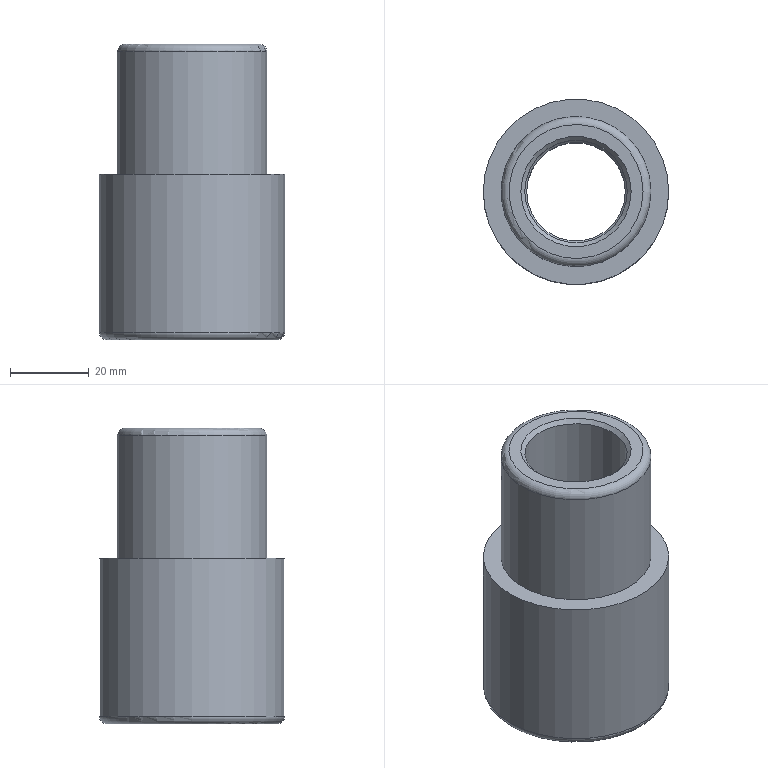Part | NX | features DATUM_CSYS 5, EXTRUDE 4, SKETCH 4, CHAMFER 2, BLEND 1 | 1 solid | 12 faces | box 47 x 47 x 75 mm | volume 71750 mm3 | cylinder 4 | plane 3 | torus 3 | cone 2 | commonest cylinder face diameters 25 x1 26 x1 38 x1 47 x1
STEP:
#1=CARTESIAN_POINT('',(12.5,0.,2.));
#2=VERTEX_POINT('',#1);
#3=CARTESIAN_POINT('',(0.,0.,2.));
#4=DIRECTION('',(0.,0.,1.));
#5=DIRECTION('',(1.,0.,0.));
#6=AXIS2_PLACEMENT_3D('',#3,#4,#5);
#7=CIRCLE('',#6,12.5);
#8=EDGE_CURVE('',#2,#2,#7,.F.);
#9=ORIENTED_EDGE('',*,*,#8,.T.);
#10=EDGE_LOOP('',(#9));
#11=FACE_BOUND('',#10,.T.);
#12=CARTESIAN_POINT('',(12.5,0.,40.));
#13=VERTEX_POINT('',#12);
#14=CARTESIAN_POINT('',(0.,0.,40.));
#15=DIRECTION('',(0.,0.,1.));
#16=DIRECTION('',(1.,0.,0.));
#17=AXIS2_PLACEMENT_3D('',#14,#15,#16);
#18=CIRCLE('',#17,12.5);
#19=EDGE_CURVE('',#13,#13,#18,.T.);
#20=ORIENTED_EDGE('',*,*,#19,.T.);
#21=EDGE_LOOP('',(#20));
#22=FACE_BOUND('',#21,.T.);
#23=CARTESIAN_POINT('',(0.,0.,-7.5));
#24=DIRECTION('',(0.,0.,1.));
#25=DIRECTION('',(1.,0.,0.));
#26=AXIS2_PLACEMENT_3D('',#23,#24,#25);
#27=CYLINDRICAL_SURFACE('',#26,12.5);
#28=ADVANCED_FACE('',(#11,#22),#27,.F.);
#29=CARTESIAN_POINT('',(23.5,0.,2.));
#30=VERTEX_POINT('',#29);
#31=CARTESIAN_POINT('',(0.,0.,2.));
#32=DIRECTION('',(0.,0.,1.));
#33=DIRECTION('',(1.,0.,0.));
#34=AXIS2_PLACEMENT_3D('',#31,#32,#33);
#35=CIRCLE('',#34,23.5);
#36=EDGE_CURVE('',#30,#30,#35,.T.);
#37=ORIENTED_EDGE('',*,*,#36,.T.);
#38=EDGE_LOOP('',(#37));
#39=FACE_BOUND('',#38,.T.);
#40=CARTESIAN_POINT('',(23.5,0.,42.));
#41=VERTEX_POINT('',#40);
#42=CARTESIAN_POINT('',(0.,0.,42.));
#43=DIRECTION('',(0.,0.,1.));
#44=DIRECTION('',(1.,0.,0.));
#45=AXIS2_PLACEMENT_3D('',#42,#43,#44);
#46=CIRCLE('',#45,23.5);
#47=EDGE_CURVE('',#41,#41,#46,.T.);
#48=ORIENTED_EDGE('',*,*,#47,.F.);
#49=EDGE_LOOP('',(#48));
#50=FACE_BOUND('',#49,.T.);
#51=CARTESIAN_POINT('',(0.,0.,42.));
#52=DIRECTION('',(0.,0.,-1.));
#53=DIRECTION('',(-1.,0.,0.));
#54=AXIS2_PLACEMENT_3D('',#51,#52,#53);
#55=CYLINDRICAL_SURFACE('',#54,23.5);
#56=ADVANCED_FACE('',(#39,#50),#55,.T.);
#57=CARTESIAN_POINT('',(19.,0.,42.));
#58=VERTEX_POINT('',#57);
#59=CARTESIAN_POINT('',(0.,0.,42.));
#60=DIRECTION('',(0.,0.,1.));
#61=DIRECTION('',(1.,0.,0.));
#62=AXIS2_PLACEMENT_3D('',#59,#60,#61);
#63=CIRCLE('',#62,19.);
#64=EDGE_CURVE('',#58,#58,#63,.T.);
#65=ORIENTED_EDGE('',*,*,#64,.F.);
#66=EDGE_LOOP('',(#65));
#67=FACE_BOUND('',#66,.T.);
#68=ORIENTED_EDGE('',*,*,#47,.T.);
#69=EDGE_LOOP('',(#68));
#70=FACE_BOUND('',#69,.T.);
#71=CARTESIAN_POINT('',(0.,0.,42.));
#72=DIRECTION('',(0.,0.,1.));
#73=DIRECTION('',(1.,0.,0.));
#74=AXIS2_PLACEMENT_3D('',#71,#72,#73);
#75=PLANE('',#74);
#76=ADVANCED_FACE('',(#67,#70),#75,.T.);
#77=CARTESIAN_POINT('',(14.5,0.,0.));
#78=VERTEX_POINT('',#77);
#79=CARTESIAN_POINT('',(0.,0.,0.));
#80=DIRECTION('',(0.,0.,1.));
#81=DIRECTION('',(1.,0.,0.));
#82=AXIS2_PLACEMENT_3D('',#79,#80,#81);
#83=CIRCLE('',#82,14.5);
#84=EDGE_CURVE('',#78,#78,#83,.T.);
#85=ORIENTED_EDGE('',*,*,#84,.T.);
#86=EDGE_LOOP('',(#85));
#87=FACE_BOUND('',#86,.T.);
#88=CARTESIAN_POINT('',(21.5,0.,0.));
#89=VERTEX_POINT('',#88);
#90=CARTESIAN_POINT('',(0.,0.,0.));
#91=DIRECTION('',(0.,0.,1.));
#92=DIRECTION('',(1.,0.,0.));
#93=AXIS2_PLACEMENT_3D('',#90,#91,#92);
#94=CIRCLE('',#93,21.5);
#95=EDGE_CURVE('',#89,#89,#94,.F.);
#96=ORIENTED_EDGE('',*,*,#95,.T.);
#97=EDGE_LOOP('',(#96));
#98=FACE_BOUND('',#97,.T.);
#99=CARTESIAN_POINT('',(0.,0.,0.));
#100=DIRECTION('',(0.,0.,1.));
#101=DIRECTION('',(1.,0.,0.));
#102=AXIS2_PLACEMENT_3D('',#99,#100,#101);
#103=PLANE('',#102);
#104=ADVANCED_FACE('',(#87,#98),#103,.F.);
#105=CARTESIAN_POINT('',(19.,0.,73.));
#106=VERTEX_POINT('',#105);
#107=CARTESIAN_POINT('',(0.,0.,73.));
#108=DIRECTION('',(0.,0.,1.));
#109=DIRECTION('',(1.,0.,0.));
#110=AXIS2_PLACEMENT_3D('',#107,#108,#109);
#111=CIRCLE('',#110,19.);
#112=EDGE_CURVE('',#106,#106,#111,.F.);
#113=ORIENTED_EDGE('',*,*,#112,.T.);
#114=EDGE_LOOP('',(#113));
#115=FACE_BOUND('',#114,.T.);
#116=ORIENTED_EDGE('',*,*,#64,.T.);
#117=EDGE_LOOP('',(#116));
#118=FACE_BOUND('',#117,.T.);
#119=CARTESIAN_POINT('',(0.,0.,75.));
#120=DIRECTION('',(0.,0.,-1.));
#121=DIRECTION('',(-1.,0.,0.));
#122=AXIS2_PLACEMENT_3D('',#119,#120,#121);
#123=CYLINDRICAL_SURFACE('',#122,19.);
#124=ADVANCED_FACE('',(#115,#118),#123,.T.);
#125=CARTESIAN_POINT('',(17.,0.,75.));
#126=VERTEX_POINT('',#125);
#127=CARTESIAN_POINT('',(0.,0.,75.));
#128=DIRECTION('',(0.,0.,1.));
#129=DIRECTION('',(1.,0.,0.));
#130=AXIS2_PLACEMENT_3D('',#127,#128,#129);
#131=CIRCLE('',#130,17.);
#132=EDGE_CURVE('',#126,#126,#131,.T.);
#133=ORIENTED_EDGE('',*,*,#132,.T.);
#134=EDGE_LOOP('',(#133));
#135=FACE_BOUND('',#134,.T.);
#136=CARTESIAN_POINT('',(14.,0.,75.));
#137=VERTEX_POINT('',#136);
#138=CARTESIAN_POINT('',(0.,0.,75.));
#139=DIRECTION('',(0.,0.,1.));
#140=DIRECTION('',(1.,0.,0.));
#141=AXIS2_PLACEMENT_3D('',#138,#139,#140);
#142=CIRCLE('',#141,14.);
#143=EDGE_CURVE('',#137,#137,#142,.F.);
#144=ORIENTED_EDGE('',*,*,#143,.T.);
#145=EDGE_LOOP('',(#144));
#146=FACE_BOUND('',#145,.T.);
#147=CARTESIAN_POINT('',(0.,0.,75.));
#148=DIRECTION('',(0.,0.,1.));
#149=DIRECTION('',(1.,0.,0.));
#150=AXIS2_PLACEMENT_3D('',#147,#148,#149);
#151=PLANE('',#150);
#152=ADVANCED_FACE('',(#135,#146),#151,.T.);
#153=CARTESIAN_POINT('',(13.,0.,74.));
#154=VERTEX_POINT('',#153);
#155=CARTESIAN_POINT('',(0.,0.,74.));
#156=DIRECTION('',(0.,0.,1.));
#157=DIRECTION('',(1.,0.,0.));
#158=AXIS2_PLACEMENT_3D('',#155,#156,#157);
#159=CIRCLE('',#158,13.);
#160=EDGE_CURVE('',#154,#154,#159,.T.);
#161=ORIENTED_EDGE('',*,*,#160,.T.);
#162=EDGE_LOOP('',(#161));
#163=FACE_BOUND('',#162,.T.);
#164=CARTESIAN_POINT('',(13.,0.,40.5));
#165=VERTEX_POINT('',#164);
#166=CARTESIAN_POINT('',(0.,0.,40.5));
#167=DIRECTION('',(0.,0.,1.));
#168=DIRECTION('',(1.,0.,0.));
#169=AXIS2_PLACEMENT_3D('',#166,#167,#168);
#170=CIRCLE('',#169,13.);
#171=EDGE_CURVE('',#165,#165,#170,.F.);
#172=ORIENTED_EDGE('',*,*,#171,.T.);
#173=EDGE_LOOP('',(#172));
#174=FACE_BOUND('',#173,.T.);
#175=CARTESIAN_POINT('',(0.,0.,40.5));
#176=DIRECTION('',(0.,0.,1.));
#177=DIRECTION('',(1.,0.,0.));
#178=AXIS2_PLACEMENT_3D('',#175,#176,#177);
#179=CYLINDRICAL_SURFACE('',#178,13.);
#180=ADVANCED_FACE('',(#163,#174),#179,.F.);
#181=ORIENTED_EDGE('',*,*,#143,.F.);
#182=EDGE_LOOP('',(#181));
#183=FACE_BOUND('',#182,.T.);
#184=ORIENTED_EDGE('',*,*,#160,.F.);
#185=EDGE_LOOP('',(#184));
#186=FACE_BOUND('',#185,.T.);
#187=CARTESIAN_POINT('',(0.,0.,74.));
#188=DIRECTION('',(0.,0.,1.));
#189=DIRECTION('',(1.,0.,0.));
#190=AXIS2_PLACEMENT_3D('',#187,#188,#189);
#191=CONICAL_SURFACE('',#190,13.,0.7854);
#192=ADVANCED_FACE('',(#183,#186),#191,.F.);
#193=ORIENTED_EDGE('',*,*,#19,.F.);
#194=EDGE_LOOP('',(#193));
#195=FACE_BOUND('',#194,.T.);
#196=ORIENTED_EDGE('',*,*,#171,.F.);
#197=EDGE_LOOP('',(#196));
#198=FACE_BOUND('',#197,.T.);
#199=CARTESIAN_POINT('',(0.,0.,40.5));
#200=DIRECTION('',(0.,0.,1.));
#201=DIRECTION('',(1.,0.,0.));
#202=AXIS2_PLACEMENT_3D('',#199,#200,#201);
#203=CONICAL_SURFACE('',#202,13.,0.7854);
#204=ADVANCED_FACE('',(#195,#198),#203,.F.);
#205=ORIENTED_EDGE('',*,*,#8,.F.);
#206=EDGE_LOOP('',(#205));
#207=FACE_BOUND('',#206,.T.);
#208=ORIENTED_EDGE('',*,*,#84,.F.);
#209=EDGE_LOOP('',(#208));
#210=FACE_BOUND('',#209,.T.);
#211=CARTESIAN_POINT('',(0.,0.,2.));
#212=DIRECTION('',(0.,0.,1.));
#213=DIRECTION('',(1.,0.,0.));
#214=AXIS2_PLACEMENT_3D('',#211,#212,#213);
#215=TOROIDAL_SURFACE('',#214,14.5,2.);
#216=ADVANCED_FACE('',(#207,#210),#215,.T.);
#217=ORIENTED_EDGE('',*,*,#95,.F.);
#218=EDGE_LOOP('',(#217));
#219=FACE_BOUND('',#218,.T.);
#220=ORIENTED_EDGE('',*,*,#36,.F.);
#221=EDGE_LOOP('',(#220));
#222=FACE_BOUND('',#221,.T.);
#223=CARTESIAN_POINT('',(0.,0.,2.));
#224=DIRECTION('',(0.,0.,1.));
#225=DIRECTION('',(1.,0.,0.));
#226=AXIS2_PLACEMENT_3D('',#223,#224,#225);
#227=TOROIDAL_SURFACE('',#226,21.5,2.);
#228=ADVANCED_FACE('',(#219,#222),#227,.T.);
#229=ORIENTED_EDGE('',*,*,#112,.F.);
#230=EDGE_LOOP('',(#229));
#231=FACE_BOUND('',#230,.T.);
#232=ORIENTED_EDGE('',*,*,#132,.F.);
#233=EDGE_LOOP('',(#232));
#234=FACE_BOUND('',#233,.T.);
#235=CARTESIAN_POINT('',(0.,0.,73.));
#236=DIRECTION('',(0.,0.,1.));
#237=DIRECTION('',(1.,0.,0.));
#238=AXIS2_PLACEMENT_3D('',#235,#236,#237);
#239=TOROIDAL_SURFACE('',#238,17.,2.);
#240=ADVANCED_FACE('',(#231,#234),#239,.T.);
#241=CLOSED_SHELL('',(#28,#56,#76,#104,#124,#152,#180,#192,#204,#216,#228,#240));
#242=MANIFOLD_SOLID_BREP('',#241);
#243=(LENGTH_UNIT()NAMED_UNIT(*)SI_UNIT(.MILLI.,.METRE.));
#244=UNCERTAINTY_MEASURE_WITH_UNIT(LENGTH_MEASURE(0.00001),#243,'','');
#245=(NAMED_UNIT(*)PLANE_ANGLE_UNIT()SI_UNIT($,.RADIAN.));
#246=(NAMED_UNIT(*)SI_UNIT($,.STERADIAN.)SOLID_ANGLE_UNIT());
#247=(GEOMETRIC_REPRESENTATION_CONTEXT(3)GLOBAL_UNCERTAINTY_ASSIGNED_CONTEXT((#244))GLOBAL_UNIT_ASSIGNED_CONTEXT((#243,#245,#246))REPRESENTATION_CONTEXT('',''));
#248=ADVANCED_BREP_SHAPE_REPRESENTATION('',(#242),#247);